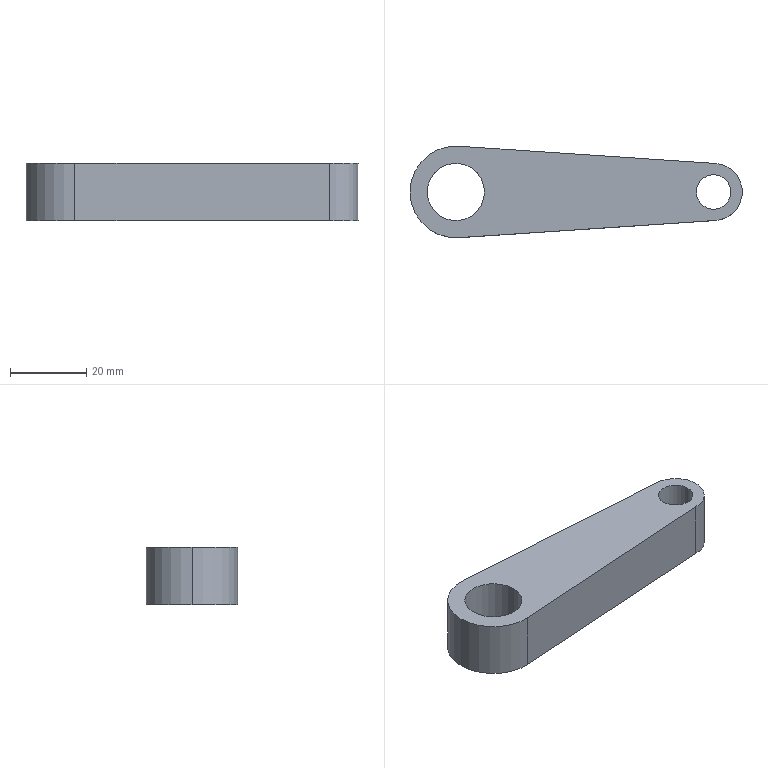Part | SolidWorks | features Extrusion 1 | 1 solid | 11 faces | box 87 x 24 x 15 mm | volume 20884 mm3 | cylinder 7 | plane 4 | commonest cylinder face diameters 15 x3 9 x2 24 x2
STEP:
#1=CARTESIAN_POINT('',(63.,0.,7.5));
#2=VERTEX_POINT('',#1);
#3=CARTESIAN_POINT('',(72.,0.,7.5));
#4=VERTEX_POINT('',#3);
#5=CARTESIAN_POINT('',(67.5,0.,7.5));
#6=DIRECTION('',(0.,0.,1.));
#7=DIRECTION('',(1.,0.,0.));
#8=AXIS2_PLACEMENT_3D('',#5,#6,#7);
#9=CIRCLE('',#8,4.5);
#10=EDGE_CURVE('',#2,#4,#9,.T.);
#11=ORIENTED_EDGE('',*,*,#10,.T.);
#12=CARTESIAN_POINT('',(72.,0.,-7.5));
#13=VERTEX_POINT('',#12);
#14=CARTESIAN_POINT('',(72.,0.,7.5));
#15=DIRECTION('',(0.,0.,-1.));
#16=VECTOR('',#15,1000.);
#17=LINE('',#14,#16);
#18=EDGE_CURVE('',#4,#13,#17,.T.);
#19=ORIENTED_EDGE('',*,*,#18,.T.);
#20=CARTESIAN_POINT('',(63.,0.,-7.5));
#21=VERTEX_POINT('',#20);
#22=CARTESIAN_POINT('',(67.5,0.,-7.5));
#23=DIRECTION('',(0.,0.,1.));
#24=DIRECTION('',(1.,0.,0.));
#25=AXIS2_PLACEMENT_3D('',#22,#23,#24);
#26=CIRCLE('',#25,4.5);
#27=EDGE_CURVE('',#21,#13,#26,.T.);
#28=ORIENTED_EDGE('',*,*,#27,.F.);
#29=CARTESIAN_POINT('',(63.,0.,7.5));
#30=DIRECTION('',(0.,0.,-1.));
#31=VECTOR('',#30,1000.);
#32=LINE('',#29,#31);
#33=EDGE_CURVE('',#2,#21,#32,.T.);
#34=ORIENTED_EDGE('',*,*,#33,.F.);
#35=EDGE_LOOP('',(#11,#19,#28,#34));
#36=FACE_OUTER_BOUND('',#35,.T.);
#37=CARTESIAN_POINT('',(67.5,0.,7.5));
#38=DIRECTION('',(0.,0.,-1.));
#39=DIRECTION('',(-1.,0.,0.));
#40=AXIS2_PLACEMENT_3D('',#37,#38,#39);
#41=CYLINDRICAL_SURFACE('',#40,4.5);
#42=ADVANCED_FACE('',(#36),#41,.F.);
#43=CARTESIAN_POINT('',(-7.5,0.,7.5));
#44=VERTEX_POINT('',#43);
#45=CARTESIAN_POINT('',(7.5,0.,7.5));
#46=VERTEX_POINT('',#45);
#47=CARTESIAN_POINT('',(0.,0.,7.5));
#48=DIRECTION('',(0.,0.,1.));
#49=DIRECTION('',(1.,0.,0.));
#50=AXIS2_PLACEMENT_3D('',#47,#48,#49);
#51=CIRCLE('',#50,7.5);
#52=EDGE_CURVE('',#44,#46,#51,.T.);
#53=ORIENTED_EDGE('',*,*,#52,.T.);
#54=CARTESIAN_POINT('',(7.5,0.,-7.5));
#55=VERTEX_POINT('',#54);
#56=CARTESIAN_POINT('',(7.5,0.,7.5));
#57=DIRECTION('',(0.,0.,-1.));
#58=VECTOR('',#57,1000.);
#59=LINE('',#56,#58);
#60=EDGE_CURVE('',#46,#55,#59,.T.);
#61=ORIENTED_EDGE('',*,*,#60,.T.);
#62=CARTESIAN_POINT('',(-7.5,0.,-7.5));
#63=VERTEX_POINT('',#62);
#64=CARTESIAN_POINT('',(0.,0.,-7.5));
#65=DIRECTION('',(0.,0.,1.));
#66=DIRECTION('',(1.,0.,0.));
#67=AXIS2_PLACEMENT_3D('',#64,#65,#66);
#68=CIRCLE('',#67,7.5);
#69=EDGE_CURVE('',#63,#55,#68,.T.);
#70=ORIENTED_EDGE('',*,*,#69,.F.);
#71=CARTESIAN_POINT('',(-7.5,0.,7.5));
#72=DIRECTION('',(0.,0.,-1.));
#73=VECTOR('',#72,1000.);
#74=LINE('',#71,#73);
#75=EDGE_CURVE('',#44,#63,#74,.T.);
#76=ORIENTED_EDGE('',*,*,#75,.F.);
#77=EDGE_LOOP('',(#53,#61,#70,#76));
#78=FACE_OUTER_BOUND('',#77,.T.);
#79=CARTESIAN_POINT('',(0.,0.,7.5));
#80=DIRECTION('',(0.,0.,-1.));
#81=DIRECTION('',(-1.,0.,0.));
#82=AXIS2_PLACEMENT_3D('',#79,#80,#81);
#83=CYLINDRICAL_SURFACE('',#82,7.5);
#84=ADVANCED_FACE('',(#78),#83,.F.);
#85=CARTESIAN_POINT('',(-12.,0.,7.5));
#86=VERTEX_POINT('',#85);
#87=CARTESIAN_POINT('',(0.803,-11.973,7.5));
#88=VERTEX_POINT('',#87);
#89=CARTESIAN_POINT('',(0.,0.,7.5));
#90=DIRECTION('',(0.,0.,1.));
#91=DIRECTION('',(1.,0.,0.));
#92=AXIS2_PLACEMENT_3D('',#89,#90,#91);
#93=CIRCLE('',#92,12.);
#94=EDGE_CURVE('',#86,#88,#93,.T.);
#95=ORIENTED_EDGE('',*,*,#94,.F.);
#96=CARTESIAN_POINT('',(-12.,0.,-7.5));
#97=VERTEX_POINT('',#96);
#98=CARTESIAN_POINT('',(-12.,0.,7.5));
#99=DIRECTION('',(0.,0.,-1.));
#100=VECTOR('',#99,1000.);
#101=LINE('',#98,#100);
#102=EDGE_CURVE('',#86,#97,#101,.T.);
#103=ORIENTED_EDGE('',*,*,#102,.T.);
#104=CARTESIAN_POINT('',(0.803,-11.973,-7.5));
#105=VERTEX_POINT('',#104);
#106=CARTESIAN_POINT('',(0.,0.,-7.5));
#107=DIRECTION('',(0.,0.,1.));
#108=DIRECTION('',(1.,0.,0.));
#109=AXIS2_PLACEMENT_3D('',#106,#107,#108);
#110=CIRCLE('',#109,12.);
#111=EDGE_CURVE('',#97,#105,#110,.T.);
#112=ORIENTED_EDGE('',*,*,#111,.T.);
#113=CARTESIAN_POINT('',(0.803,-11.973,7.5));
#114=DIRECTION('',(0.,0.,-1.));
#115=VECTOR('',#114,1000.);
#116=LINE('',#113,#115);
#117=EDGE_CURVE('',#88,#105,#116,.T.);
#118=ORIENTED_EDGE('',*,*,#117,.F.);
#119=EDGE_LOOP('',(#95,#103,#112,#118));
#120=FACE_OUTER_BOUND('',#119,.T.);
#121=CARTESIAN_POINT('',(0.,0.,7.5));
#122=DIRECTION('',(0.,0.,-1.));
#123=DIRECTION('',(-1.,0.,0.));
#124=AXIS2_PLACEMENT_3D('',#121,#122,#123);
#125=CYLINDRICAL_SURFACE('',#124,12.);
#126=ADVANCED_FACE('',(#120),#125,.T.);
#127=ORIENTED_EDGE('',*,*,#52,.F.);
#128=CARTESIAN_POINT('',(0.,0.,7.5));
#129=DIRECTION('',(0.,0.,1.));
#130=DIRECTION('',(1.,0.,0.));
#131=AXIS2_PLACEMENT_3D('',#128,#129,#130);
#132=CIRCLE('',#131,7.5);
#133=EDGE_CURVE('',#46,#44,#132,.T.);
#134=ORIENTED_EDGE('',*,*,#133,.F.);
#135=EDGE_LOOP('',(#127,#134));
#136=FACE_BOUND('',#135,.T.);
#137=CARTESIAN_POINT('',(0.803,11.973,7.5));
#138=VERTEX_POINT('',#137);
#139=CARTESIAN_POINT('',(0.,0.,7.5));
#140=DIRECTION('',(0.,0.,1.));
#141=DIRECTION('',(1.,0.,0.));
#142=AXIS2_PLACEMENT_3D('',#139,#140,#141);
#143=CIRCLE('',#142,12.);
#144=EDGE_CURVE('',#138,#86,#143,.T.);
#145=ORIENTED_EDGE('',*,*,#144,.T.);
#146=ORIENTED_EDGE('',*,*,#94,.T.);
#147=CARTESIAN_POINT('',(67.5,-7.5,7.5));
#148=VERTEX_POINT('',#147);
#149=CARTESIAN_POINT('',(0.803,-11.973,7.5));
#150=DIRECTION('',(0.9978,0.06692,0.));
#151=VECTOR('',#150,1000.);
#152=LINE('',#149,#151);
#153=EDGE_CURVE('',#88,#148,#152,.T.);
#154=ORIENTED_EDGE('',*,*,#153,.T.);
#155=CARTESIAN_POINT('',(67.5,7.5,7.5));
#156=VERTEX_POINT('',#155);
#157=CARTESIAN_POINT('',(67.5,0.,7.5));
#158=DIRECTION('',(0.,0.,1.));
#159=DIRECTION('',(1.,0.,0.));
#160=AXIS2_PLACEMENT_3D('',#157,#158,#159);
#161=CIRCLE('',#160,7.5);
#162=EDGE_CURVE('',#148,#156,#161,.T.);
#163=ORIENTED_EDGE('',*,*,#162,.T.);
#164=CARTESIAN_POINT('',(0.803,11.973,7.5));
#165=DIRECTION('',(-0.9978,0.06692,0.));
#166=VECTOR('',#165,1000.);
#167=LINE('',#164,#166);
#168=EDGE_CURVE('',#156,#138,#167,.T.);
#169=ORIENTED_EDGE('',*,*,#168,.T.);
#170=EDGE_LOOP('',(#145,#146,#154,#163,#169));
#171=FACE_OUTER_BOUND('',#170,.T.);
#172=ORIENTED_EDGE('',*,*,#10,.F.);
#173=CARTESIAN_POINT('',(67.5,0.,7.5));
#174=DIRECTION('',(0.,0.,1.));
#175=DIRECTION('',(1.,0.,0.));
#176=AXIS2_PLACEMENT_3D('',#173,#174,#175);
#177=CIRCLE('',#176,4.5);
#178=EDGE_CURVE('',#4,#2,#177,.T.);
#179=ORIENTED_EDGE('',*,*,#178,.F.);
#180=EDGE_LOOP('',(#172,#179));
#181=FACE_BOUND('',#180,.T.);
#182=CARTESIAN_POINT('',(0.,0.,7.5));
#183=DIRECTION('',(0.,0.,1.));
#184=DIRECTION('',(1.,0.,0.));
#185=AXIS2_PLACEMENT_3D('',#182,#183,#184);
#186=PLANE('',#185);
#187=ADVANCED_FACE('',(#136,#171,#181),#186,.T.);
#188=CARTESIAN_POINT('',(0.803,11.973,-7.5));
#189=VERTEX_POINT('',#188);
#190=CARTESIAN_POINT('',(0.,0.,-7.5));
#191=DIRECTION('',(0.,0.,1.));
#192=DIRECTION('',(1.,0.,0.));
#193=AXIS2_PLACEMENT_3D('',#190,#191,#192);
#194=CIRCLE('',#193,12.);
#195=EDGE_CURVE('',#189,#97,#194,.T.);
#196=ORIENTED_EDGE('',*,*,#195,.F.);
#197=CARTESIAN_POINT('',(67.5,7.5,-7.5));
#198=VERTEX_POINT('',#197);
#199=CARTESIAN_POINT('',(0.803,11.973,-7.5));
#200=DIRECTION('',(-0.9978,0.06692,0.));
#201=VECTOR('',#200,1000.);
#202=LINE('',#199,#201);
#203=EDGE_CURVE('',#198,#189,#202,.T.);
#204=ORIENTED_EDGE('',*,*,#203,.F.);
#205=CARTESIAN_POINT('',(67.5,-7.5,-7.5));
#206=VERTEX_POINT('',#205);
#207=CARTESIAN_POINT('',(67.5,0.,-7.5));
#208=DIRECTION('',(0.,0.,1.));
#209=DIRECTION('',(1.,0.,0.));
#210=AXIS2_PLACEMENT_3D('',#207,#208,#209);
#211=CIRCLE('',#210,7.5);
#212=EDGE_CURVE('',#206,#198,#211,.T.);
#213=ORIENTED_EDGE('',*,*,#212,.F.);
#214=CARTESIAN_POINT('',(0.803,-11.973,-7.5));
#215=DIRECTION('',(0.9978,0.06692,0.));
#216=VECTOR('',#215,1000.);
#217=LINE('',#214,#216);
#218=EDGE_CURVE('',#105,#206,#217,.T.);
#219=ORIENTED_EDGE('',*,*,#218,.F.);
#220=ORIENTED_EDGE('',*,*,#111,.F.);
#221=EDGE_LOOP('',(#196,#204,#213,#219,#220));
#222=FACE_OUTER_BOUND('',#221,.T.);
#223=ORIENTED_EDGE('',*,*,#69,.T.);
#224=CARTESIAN_POINT('',(0.,0.,-7.5));
#225=DIRECTION('',(0.,0.,1.));
#226=DIRECTION('',(1.,0.,0.));
#227=AXIS2_PLACEMENT_3D('',#224,#225,#226);
#228=CIRCLE('',#227,7.5);
#229=EDGE_CURVE('',#55,#63,#228,.T.);
#230=ORIENTED_EDGE('',*,*,#229,.T.);
#231=EDGE_LOOP('',(#223,#230));
#232=FACE_BOUND('',#231,.T.);
#233=ORIENTED_EDGE('',*,*,#27,.T.);
#234=CARTESIAN_POINT('',(67.5,0.,-7.5));
#235=DIRECTION('',(0.,0.,1.));
#236=DIRECTION('',(1.,0.,0.));
#237=AXIS2_PLACEMENT_3D('',#234,#235,#236);
#238=CIRCLE('',#237,4.5);
#239=EDGE_CURVE('',#13,#21,#238,.T.);
#240=ORIENTED_EDGE('',*,*,#239,.T.);
#241=EDGE_LOOP('',(#233,#240));
#242=FACE_BOUND('',#241,.T.);
#243=CARTESIAN_POINT('',(0.,0.,-7.5));
#244=DIRECTION('',(0.,0.,1.));
#245=DIRECTION('',(1.,0.,0.));
#246=AXIS2_PLACEMENT_3D('',#243,#244,#245);
#247=PLANE('',#246);
#248=ADVANCED_FACE('',(#222,#232,#242),#247,.F.);
#249=ORIENTED_EDGE('',*,*,#102,.F.);
#250=ORIENTED_EDGE('',*,*,#144,.F.);
#251=CARTESIAN_POINT('',(0.803,11.973,7.5));
#252=DIRECTION('',(0.,0.,-1.));
#253=VECTOR('',#252,1000.);
#254=LINE('',#251,#253);
#255=EDGE_CURVE('',#138,#189,#254,.T.);
#256=ORIENTED_EDGE('',*,*,#255,.T.);
#257=ORIENTED_EDGE('',*,*,#195,.T.);
#258=EDGE_LOOP('',(#249,#250,#256,#257));
#259=FACE_OUTER_BOUND('',#258,.T.);
#260=CARTESIAN_POINT('',(0.,0.,7.5));
#261=DIRECTION('',(0.,0.,-1.));
#262=DIRECTION('',(-1.,0.,0.));
#263=AXIS2_PLACEMENT_3D('',#260,#261,#262);
#264=CYLINDRICAL_SURFACE('',#263,12.);
#265=ADVANCED_FACE('',(#259),#264,.T.);
#266=ORIENTED_EDGE('',*,*,#218,.T.);
#267=CARTESIAN_POINT('',(67.5,-7.5,7.5));
#268=DIRECTION('',(0.,0.,-1.));
#269=VECTOR('',#268,1000.);
#270=LINE('',#267,#269);
#271=EDGE_CURVE('',#148,#206,#270,.T.);
#272=ORIENTED_EDGE('',*,*,#271,.F.);
#273=ORIENTED_EDGE('',*,*,#153,.F.);
#274=ORIENTED_EDGE('',*,*,#117,.T.);
#275=EDGE_LOOP('',(#266,#272,#273,#274));
#276=FACE_OUTER_BOUND('',#275,.T.);
#277=CARTESIAN_POINT('',(0.803,-11.973,7.5));
#278=DIRECTION('',(-0.06692,0.9978,0.));
#279=DIRECTION('',(-0.9978,-0.06692,0.));
#280=AXIS2_PLACEMENT_3D('',#277,#278,#279);
#281=PLANE('',#280);
#282=ADVANCED_FACE('',(#276),#281,.F.);
#283=ORIENTED_EDGE('',*,*,#212,.T.);
#284=CARTESIAN_POINT('',(67.5,7.5,7.5));
#285=DIRECTION('',(0.,0.,-1.));
#286=VECTOR('',#285,1000.);
#287=LINE('',#284,#286);
#288=EDGE_CURVE('',#156,#198,#287,.T.);
#289=ORIENTED_EDGE('',*,*,#288,.F.);
#290=ORIENTED_EDGE('',*,*,#162,.F.);
#291=ORIENTED_EDGE('',*,*,#271,.T.);
#292=EDGE_LOOP('',(#283,#289,#290,#291));
#293=FACE_OUTER_BOUND('',#292,.T.);
#294=CARTESIAN_POINT('',(67.5,0.,7.5));
#295=DIRECTION('',(0.,0.,-1.));
#296=DIRECTION('',(-1.,0.,0.));
#297=AXIS2_PLACEMENT_3D('',#294,#295,#296);
#298=CYLINDRICAL_SURFACE('',#297,7.5);
#299=ADVANCED_FACE('',(#293),#298,.T.);
#300=ORIENTED_EDGE('',*,*,#203,.T.);
#301=ORIENTED_EDGE('',*,*,#255,.F.);
#302=ORIENTED_EDGE('',*,*,#168,.F.);
#303=ORIENTED_EDGE('',*,*,#288,.T.);
#304=EDGE_LOOP('',(#300,#301,#302,#303));
#305=FACE_OUTER_BOUND('',#304,.T.);
#306=CARTESIAN_POINT('',(0.803,11.973,7.5));
#307=DIRECTION('',(-0.06692,-0.9978,0.));
#308=DIRECTION('',(0.9978,-0.06692,0.));
#309=AXIS2_PLACEMENT_3D('',#306,#307,#308);
#310=PLANE('',#309);
#311=ADVANCED_FACE('',(#305),#310,.F.);
#312=ORIENTED_EDGE('',*,*,#60,.F.);
#313=ORIENTED_EDGE('',*,*,#133,.T.);
#314=ORIENTED_EDGE('',*,*,#75,.T.);
#315=ORIENTED_EDGE('',*,*,#229,.F.);
#316=EDGE_LOOP('',(#312,#313,#314,#315));
#317=FACE_OUTER_BOUND('',#316,.T.);
#318=CARTESIAN_POINT('',(0.,0.,7.5));
#319=DIRECTION('',(0.,0.,-1.));
#320=DIRECTION('',(-1.,0.,0.));
#321=AXIS2_PLACEMENT_3D('',#318,#319,#320);
#322=CYLINDRICAL_SURFACE('',#321,7.5);
#323=ADVANCED_FACE('',(#317),#322,.F.);
#324=ORIENTED_EDGE('',*,*,#18,.F.);
#325=ORIENTED_EDGE('',*,*,#178,.T.);
#326=ORIENTED_EDGE('',*,*,#33,.T.);
#327=ORIENTED_EDGE('',*,*,#239,.F.);
#328=EDGE_LOOP('',(#324,#325,#326,#327));
#329=FACE_OUTER_BOUND('',#328,.T.);
#330=CARTESIAN_POINT('',(67.5,0.,7.5));
#331=DIRECTION('',(0.,0.,-1.));
#332=DIRECTION('',(-1.,0.,0.));
#333=AXIS2_PLACEMENT_3D('',#330,#331,#332);
#334=CYLINDRICAL_SURFACE('',#333,4.5);
#335=ADVANCED_FACE('',(#329),#334,.F.);
#336=CLOSED_SHELL('',(#42,#84,#126,#187,#248,#265,#282,#299,#311,#323,#335));
#337=MANIFOLD_SOLID_BREP('',#336);
#338=CARTESIAN_POINT('',(0.,0.,0.));
#339=DIRECTION('',(0.,0.,1.));
#340=DIRECTION('',(1.,0.,0.));
#341=AXIS2_PLACEMENT_3D('',#338,#339,#340);
#342=(LENGTH_UNIT()NAMED_UNIT(*)SI_UNIT(.MILLI.,.METRE.));
#343=UNCERTAINTY_MEASURE_WITH_UNIT(LENGTH_MEASURE(0.00001),#342,'','');
#344=(NAMED_UNIT(*)PLANE_ANGLE_UNIT()SI_UNIT($,.RADIAN.));
#345=(NAMED_UNIT(*)SI_UNIT($,.STERADIAN.)SOLID_ANGLE_UNIT());
#346=(GEOMETRIC_REPRESENTATION_CONTEXT(3)GLOBAL_UNCERTAINTY_ASSIGNED_CONTEXT((#343))GLOBAL_UNIT_ASSIGNED_CONTEXT((#342,#344,#345))REPRESENTATION_CONTEXT('',''));
#347=ADVANCED_BREP_SHAPE_REPRESENTATION('',(#337,#341),#346);